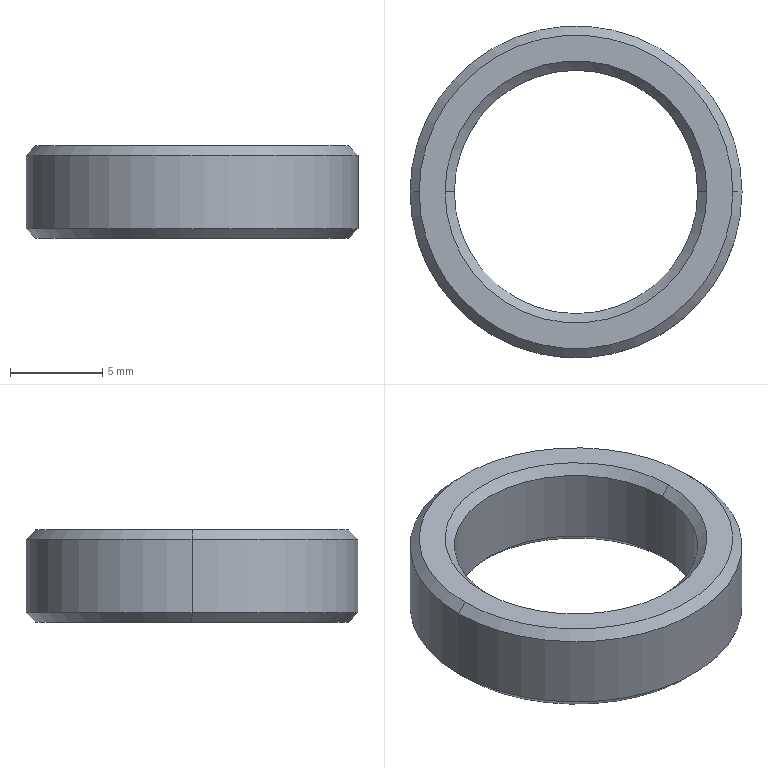Part | STEP file | 229H151427 Default | 1 solid | 14 faces | box 18 x 18 x 5 mm | volume 563.602 mm3 | cone 8 | cylinder 4 | plane 2 | commonest cylinder face diameters 13.2 x2 18 x2
STEP:
#1=CARTESIAN_POINT('',(-6.6,0.,4.5));
#2=VERTEX_POINT('',#1);
#3=CARTESIAN_POINT('',(6.6,0.,4.5));
#4=VERTEX_POINT('',#3);
#5=CARTESIAN_POINT('',(0.,0.,4.5));
#6=DIRECTION('',(0.,0.,1.));
#7=DIRECTION('',(1.,0.,0.));
#8=AXIS2_PLACEMENT_3D('',#5,#6,#7);
#9=CIRCLE('',#8,6.6);
#10=EDGE_CURVE('',#2,#4,#9,.T.);
#11=ORIENTED_EDGE('',*,*,#10,.F.);
#12=CARTESIAN_POINT('',(-7.1,0.,5.));
#13=VERTEX_POINT('',#12);
#14=CARTESIAN_POINT('',(-6.6,0.,4.5));
#15=DIRECTION('',(-0.7071,0.,0.7071));
#16=VECTOR('',#15,1000.);
#17=LINE('',#14,#16);
#18=EDGE_CURVE('',#2,#13,#17,.T.);
#19=ORIENTED_EDGE('',*,*,#18,.T.);
#20=CARTESIAN_POINT('',(7.1,0.,5.));
#21=VERTEX_POINT('',#20);
#22=CARTESIAN_POINT('',(0.,0.,5.));
#23=DIRECTION('',(0.,0.,-1.));
#24=DIRECTION('',(1.,0.,0.));
#25=AXIS2_PLACEMENT_3D('',#22,#23,#24);
#26=CIRCLE('',#25,7.1);
#27=EDGE_CURVE('',#21,#13,#26,.T.);
#28=ORIENTED_EDGE('',*,*,#27,.F.);
#29=CARTESIAN_POINT('',(6.6,0.,4.5));
#30=DIRECTION('',(0.7071,0.,0.7071));
#31=VECTOR('',#30,1000.);
#32=LINE('',#29,#31);
#33=EDGE_CURVE('',#4,#21,#32,.T.);
#34=ORIENTED_EDGE('',*,*,#33,.F.);
#35=EDGE_LOOP('',(#11,#19,#28,#34));
#36=FACE_OUTER_BOUND('',#35,.T.);
#37=CARTESIAN_POINT('',(0.,0.,4.5));
#38=DIRECTION('',(0.,0.,1.));
#39=DIRECTION('',(1.,0.,0.));
#40=AXIS2_PLACEMENT_3D('',#37,#38,#39);
#41=CONICAL_SURFACE('',#40,6.6,0.7854);
#42=ADVANCED_FACE('',(#36),#41,.F.);
#43=CARTESIAN_POINT('',(6.6,0.,0.5));
#44=VERTEX_POINT('',#43);
#45=CARTESIAN_POINT('',(-6.6,0.,0.5));
#46=VERTEX_POINT('',#45);
#47=CARTESIAN_POINT('',(0.,0.,0.5));
#48=DIRECTION('',(0.,0.,-1.));
#49=DIRECTION('',(1.,0.,0.));
#50=AXIS2_PLACEMENT_3D('',#47,#48,#49);
#51=CIRCLE('',#50,6.6);
#52=EDGE_CURVE('',#44,#46,#51,.T.);
#53=ORIENTED_EDGE('',*,*,#52,.F.);
#54=CARTESIAN_POINT('',(7.1,0.,0.));
#55=VERTEX_POINT('',#54);
#56=CARTESIAN_POINT('',(7.1,0.,0.));
#57=DIRECTION('',(0.7071,0.,-0.7071));
#58=VECTOR('',#57,1000.);
#59=LINE('',#56,#58);
#60=EDGE_CURVE('',#44,#55,#59,.T.);
#61=ORIENTED_EDGE('',*,*,#60,.T.);
#62=CARTESIAN_POINT('',(-7.1,0.,0.));
#63=VERTEX_POINT('',#62);
#64=CARTESIAN_POINT('',(0.,0.,0.));
#65=DIRECTION('',(0.,0.,1.));
#66=DIRECTION('',(1.,0.,0.));
#67=AXIS2_PLACEMENT_3D('',#64,#65,#66);
#68=CIRCLE('',#67,7.1);
#69=EDGE_CURVE('',#63,#55,#68,.T.);
#70=ORIENTED_EDGE('',*,*,#69,.F.);
#71=CARTESIAN_POINT('',(-7.1,0.,0.));
#72=DIRECTION('',(-0.7071,0.,-0.7071));
#73=VECTOR('',#72,1000.);
#74=LINE('',#71,#73);
#75=EDGE_CURVE('',#46,#63,#74,.T.);
#76=ORIENTED_EDGE('',*,*,#75,.F.);
#77=EDGE_LOOP('',(#53,#61,#70,#76));
#78=FACE_OUTER_BOUND('',#77,.T.);
#79=CARTESIAN_POINT('',(0.,0.,0.));
#80=DIRECTION('',(0.,0.,-1.));
#81=DIRECTION('',(-1.,0.,0.));
#82=AXIS2_PLACEMENT_3D('',#79,#80,#81);
#83=CONICAL_SURFACE('',#82,7.1,0.7854);
#84=ADVANCED_FACE('',(#78),#83,.F.);
#85=CARTESIAN_POINT('',(8.5,0.,5.));
#86=VERTEX_POINT('',#85);
#87=CARTESIAN_POINT('',(-8.5,0.,5.));
#88=VERTEX_POINT('',#87);
#89=CARTESIAN_POINT('',(0.,0.,5.));
#90=DIRECTION('',(0.,0.,1.));
#91=DIRECTION('',(1.,0.,0.));
#92=AXIS2_PLACEMENT_3D('',#89,#90,#91);
#93=CIRCLE('',#92,8.5);
#94=EDGE_CURVE('',#86,#88,#93,.T.);
#95=ORIENTED_EDGE('',*,*,#94,.F.);
#96=CARTESIAN_POINT('',(9.,0.,4.5));
#97=VERTEX_POINT('',#96);
#98=CARTESIAN_POINT('',(8.5,0.,5.));
#99=DIRECTION('',(0.7071,0.,-0.7071));
#100=VECTOR('',#99,1000.);
#101=LINE('',#98,#100);
#102=EDGE_CURVE('',#86,#97,#101,.T.);
#103=ORIENTED_EDGE('',*,*,#102,.T.);
#104=CARTESIAN_POINT('',(-9.,0.,4.5));
#105=VERTEX_POINT('',#104);
#106=CARTESIAN_POINT('',(0.,0.,4.5));
#107=DIRECTION('',(0.,0.,-1.));
#108=DIRECTION('',(1.,0.,0.));
#109=AXIS2_PLACEMENT_3D('',#106,#107,#108);
#110=CIRCLE('',#109,9.);
#111=EDGE_CURVE('',#105,#97,#110,.T.);
#112=ORIENTED_EDGE('',*,*,#111,.F.);
#113=CARTESIAN_POINT('',(-8.5,0.,5.));
#114=DIRECTION('',(-0.7071,0.,-0.7071));
#115=VECTOR('',#114,1000.);
#116=LINE('',#113,#115);
#117=EDGE_CURVE('',#88,#105,#116,.T.);
#118=ORIENTED_EDGE('',*,*,#117,.F.);
#119=EDGE_LOOP('',(#95,#103,#112,#118));
#120=FACE_OUTER_BOUND('',#119,.T.);
#121=CARTESIAN_POINT('',(0.,0.,5.));
#122=DIRECTION('',(0.,0.,-1.));
#123=DIRECTION('',(-1.,0.,0.));
#124=AXIS2_PLACEMENT_3D('',#121,#122,#123);
#125=CONICAL_SURFACE('',#124,8.5,0.7854);
#126=ADVANCED_FACE('',(#120),#125,.T.);
#127=CARTESIAN_POINT('',(-8.5,0.,0.));
#128=VERTEX_POINT('',#127);
#129=CARTESIAN_POINT('',(8.5,0.,0.));
#130=VERTEX_POINT('',#129);
#131=CARTESIAN_POINT('',(0.,0.,0.));
#132=DIRECTION('',(0.,0.,-1.));
#133=DIRECTION('',(1.,0.,0.));
#134=AXIS2_PLACEMENT_3D('',#131,#132,#133);
#135=CIRCLE('',#134,8.5);
#136=EDGE_CURVE('',#128,#130,#135,.T.);
#137=ORIENTED_EDGE('',*,*,#136,.F.);
#138=CARTESIAN_POINT('',(-9.,0.,0.5));
#139=VERTEX_POINT('',#138);
#140=CARTESIAN_POINT('',(-9.,0.,0.5));
#141=DIRECTION('',(-0.7071,0.,0.7071));
#142=VECTOR('',#141,1000.);
#143=LINE('',#140,#142);
#144=EDGE_CURVE('',#128,#139,#143,.T.);
#145=ORIENTED_EDGE('',*,*,#144,.T.);
#146=CARTESIAN_POINT('',(9.,0.,0.5));
#147=VERTEX_POINT('',#146);
#148=CARTESIAN_POINT('',(0.,0.,0.5));
#149=DIRECTION('',(0.,0.,1.));
#150=DIRECTION('',(1.,0.,0.));
#151=AXIS2_PLACEMENT_3D('',#148,#149,#150);
#152=CIRCLE('',#151,9.);
#153=EDGE_CURVE('',#147,#139,#152,.T.);
#154=ORIENTED_EDGE('',*,*,#153,.F.);
#155=CARTESIAN_POINT('',(9.,0.,0.5));
#156=DIRECTION('',(0.7071,0.,0.7071));
#157=VECTOR('',#156,1000.);
#158=LINE('',#155,#157);
#159=EDGE_CURVE('',#130,#147,#158,.T.);
#160=ORIENTED_EDGE('',*,*,#159,.F.);
#161=EDGE_LOOP('',(#137,#145,#154,#160));
#162=FACE_OUTER_BOUND('',#161,.T.);
#163=CARTESIAN_POINT('',(0.,0.,0.5));
#164=DIRECTION('',(0.,0.,1.));
#165=DIRECTION('',(1.,0.,0.));
#166=AXIS2_PLACEMENT_3D('',#163,#164,#165);
#167=CONICAL_SURFACE('',#166,9.,0.7854);
#168=ADVANCED_FACE('',(#162),#167,.T.);
#169=ORIENTED_EDGE('',*,*,#10,.T.);
#170=CARTESIAN_POINT('',(6.6,0.,5.));
#171=DIRECTION('',(0.,0.,-1.));
#172=VECTOR('',#171,1000.);
#173=LINE('',#170,#172);
#174=EDGE_CURVE('',#4,#44,#173,.T.);
#175=ORIENTED_EDGE('',*,*,#174,.T.);
#176=ORIENTED_EDGE('',*,*,#52,.T.);
#177=CARTESIAN_POINT('',(-6.6,0.,5.));
#178=DIRECTION('',(0.,0.,-1.));
#179=VECTOR('',#178,1000.);
#180=LINE('',#177,#179);
#181=EDGE_CURVE('',#2,#46,#180,.T.);
#182=ORIENTED_EDGE('',*,*,#181,.F.);
#183=EDGE_LOOP('',(#169,#175,#176,#182));
#184=FACE_OUTER_BOUND('',#183,.T.);
#185=CARTESIAN_POINT('',(0.,0.,5.));
#186=DIRECTION('',(0.,0.,-1.));
#187=DIRECTION('',(-1.,0.,0.));
#188=AXIS2_PLACEMENT_3D('',#185,#186,#187);
#189=CYLINDRICAL_SURFACE('',#188,6.6);
#190=ADVANCED_FACE('',(#184),#189,.F.);
#191=ORIENTED_EDGE('',*,*,#111,.T.);
#192=CARTESIAN_POINT('',(9.,0.,5.));
#193=DIRECTION('',(0.,0.,-1.));
#194=VECTOR('',#193,1000.);
#195=LINE('',#192,#194);
#196=EDGE_CURVE('',#97,#147,#195,.T.);
#197=ORIENTED_EDGE('',*,*,#196,.T.);
#198=ORIENTED_EDGE('',*,*,#153,.T.);
#199=CARTESIAN_POINT('',(-9.,0.,5.));
#200=DIRECTION('',(0.,0.,-1.));
#201=VECTOR('',#200,1000.);
#202=LINE('',#199,#201);
#203=EDGE_CURVE('',#105,#139,#202,.T.);
#204=ORIENTED_EDGE('',*,*,#203,.F.);
#205=EDGE_LOOP('',(#191,#197,#198,#204));
#206=FACE_OUTER_BOUND('',#205,.T.);
#207=CARTESIAN_POINT('',(0.,0.,5.));
#208=DIRECTION('',(0.,0.,-1.));
#209=DIRECTION('',(-1.,0.,0.));
#210=AXIS2_PLACEMENT_3D('',#207,#208,#209);
#211=CYLINDRICAL_SURFACE('',#210,9.);
#212=ADVANCED_FACE('',(#206),#211,.T.);
#213=ORIENTED_EDGE('',*,*,#27,.T.);
#214=CARTESIAN_POINT('',(0.,0.,5.));
#215=DIRECTION('',(0.,0.,-1.));
#216=DIRECTION('',(1.,0.,0.));
#217=AXIS2_PLACEMENT_3D('',#214,#215,#216);
#218=CIRCLE('',#217,7.1);
#219=EDGE_CURVE('',#13,#21,#218,.T.);
#220=ORIENTED_EDGE('',*,*,#219,.T.);
#221=EDGE_LOOP('',(#213,#220));
#222=FACE_BOUND('',#221,.T.);
#223=CARTESIAN_POINT('',(0.,0.,5.));
#224=DIRECTION('',(0.,0.,1.));
#225=DIRECTION('',(1.,0.,0.));
#226=AXIS2_PLACEMENT_3D('',#223,#224,#225);
#227=CIRCLE('',#226,8.5);
#228=EDGE_CURVE('',#88,#86,#227,.T.);
#229=ORIENTED_EDGE('',*,*,#228,.T.);
#230=ORIENTED_EDGE('',*,*,#94,.T.);
#231=EDGE_LOOP('',(#229,#230));
#232=FACE_OUTER_BOUND('',#231,.T.);
#233=CARTESIAN_POINT('',(0.,0.,5.));
#234=DIRECTION('',(0.,0.,1.));
#235=DIRECTION('',(1.,0.,0.));
#236=AXIS2_PLACEMENT_3D('',#233,#234,#235);
#237=PLANE('',#236);
#238=ADVANCED_FACE('',(#222,#232),#237,.T.);
#239=ORIENTED_EDGE('',*,*,#69,.T.);
#240=CARTESIAN_POINT('',(0.,0.,0.));
#241=DIRECTION('',(0.,0.,1.));
#242=DIRECTION('',(1.,0.,0.));
#243=AXIS2_PLACEMENT_3D('',#240,#241,#242);
#244=CIRCLE('',#243,7.1);
#245=EDGE_CURVE('',#55,#63,#244,.T.);
#246=ORIENTED_EDGE('',*,*,#245,.T.);
#247=EDGE_LOOP('',(#239,#246));
#248=FACE_BOUND('',#247,.T.);
#249=CARTESIAN_POINT('',(0.,0.,0.));
#250=DIRECTION('',(0.,0.,-1.));
#251=DIRECTION('',(1.,0.,0.));
#252=AXIS2_PLACEMENT_3D('',#249,#250,#251);
#253=CIRCLE('',#252,8.5);
#254=EDGE_CURVE('',#130,#128,#253,.T.);
#255=ORIENTED_EDGE('',*,*,#254,.T.);
#256=ORIENTED_EDGE('',*,*,#136,.T.);
#257=EDGE_LOOP('',(#255,#256));
#258=FACE_OUTER_BOUND('',#257,.T.);
#259=CARTESIAN_POINT('',(0.,0.,0.));
#260=DIRECTION('',(0.,0.,1.));
#261=DIRECTION('',(1.,0.,0.));
#262=AXIS2_PLACEMENT_3D('',#259,#260,#261);
#263=PLANE('',#262);
#264=ADVANCED_FACE('',(#248,#258),#263,.F.);
#265=ORIENTED_EDGE('',*,*,#196,.F.);
#266=CARTESIAN_POINT('',(0.,0.,4.5));
#267=DIRECTION('',(0.,0.,-1.));
#268=DIRECTION('',(1.,0.,0.));
#269=AXIS2_PLACEMENT_3D('',#266,#267,#268);
#270=CIRCLE('',#269,9.);
#271=EDGE_CURVE('',#97,#105,#270,.T.);
#272=ORIENTED_EDGE('',*,*,#271,.T.);
#273=ORIENTED_EDGE('',*,*,#203,.T.);
#274=CARTESIAN_POINT('',(0.,0.,0.5));
#275=DIRECTION('',(0.,0.,1.));
#276=DIRECTION('',(1.,0.,0.));
#277=AXIS2_PLACEMENT_3D('',#274,#275,#276);
#278=CIRCLE('',#277,9.);
#279=EDGE_CURVE('',#139,#147,#278,.T.);
#280=ORIENTED_EDGE('',*,*,#279,.T.);
#281=EDGE_LOOP('',(#265,#272,#273,#280));
#282=FACE_OUTER_BOUND('',#281,.T.);
#283=CARTESIAN_POINT('',(0.,0.,5.));
#284=DIRECTION('',(0.,0.,-1.));
#285=DIRECTION('',(-1.,0.,0.));
#286=AXIS2_PLACEMENT_3D('',#283,#284,#285);
#287=CYLINDRICAL_SURFACE('',#286,9.);
#288=ADVANCED_FACE('',(#282),#287,.T.);
#289=ORIENTED_EDGE('',*,*,#174,.F.);
#290=CARTESIAN_POINT('',(0.,0.,4.5));
#291=DIRECTION('',(0.,0.,1.));
#292=DIRECTION('',(1.,0.,0.));
#293=AXIS2_PLACEMENT_3D('',#290,#291,#292);
#294=CIRCLE('',#293,6.6);
#295=EDGE_CURVE('',#4,#2,#294,.T.);
#296=ORIENTED_EDGE('',*,*,#295,.T.);
#297=ORIENTED_EDGE('',*,*,#181,.T.);
#298=CARTESIAN_POINT('',(0.,0.,0.5));
#299=DIRECTION('',(0.,0.,-1.));
#300=DIRECTION('',(1.,0.,0.));
#301=AXIS2_PLACEMENT_3D('',#298,#299,#300);
#302=CIRCLE('',#301,6.6);
#303=EDGE_CURVE('',#46,#44,#302,.T.);
#304=ORIENTED_EDGE('',*,*,#303,.T.);
#305=EDGE_LOOP('',(#289,#296,#297,#304));
#306=FACE_OUTER_BOUND('',#305,.T.);
#307=CARTESIAN_POINT('',(0.,0.,5.));
#308=DIRECTION('',(0.,0.,-1.));
#309=DIRECTION('',(-1.,0.,0.));
#310=AXIS2_PLACEMENT_3D('',#307,#308,#309);
#311=CYLINDRICAL_SURFACE('',#310,6.6);
#312=ADVANCED_FACE('',(#306),#311,.F.);
#313=ORIENTED_EDGE('',*,*,#144,.F.);
#314=ORIENTED_EDGE('',*,*,#254,.F.);
#315=ORIENTED_EDGE('',*,*,#159,.T.);
#316=ORIENTED_EDGE('',*,*,#279,.F.);
#317=EDGE_LOOP('',(#313,#314,#315,#316));
#318=FACE_OUTER_BOUND('',#317,.T.);
#319=CARTESIAN_POINT('',(0.,0.,0.5));
#320=DIRECTION('',(0.,0.,1.));
#321=DIRECTION('',(1.,0.,0.));
#322=AXIS2_PLACEMENT_3D('',#319,#320,#321);
#323=CONICAL_SURFACE('',#322,9.,0.7854);
#324=ADVANCED_FACE('',(#318),#323,.T.);
#325=ORIENTED_EDGE('',*,*,#102,.F.);
#326=ORIENTED_EDGE('',*,*,#228,.F.);
#327=ORIENTED_EDGE('',*,*,#117,.T.);
#328=ORIENTED_EDGE('',*,*,#271,.F.);
#329=EDGE_LOOP('',(#325,#326,#327,#328));
#330=FACE_OUTER_BOUND('',#329,.T.);
#331=CARTESIAN_POINT('',(0.,0.,5.));
#332=DIRECTION('',(0.,0.,-1.));
#333=DIRECTION('',(-1.,0.,0.));
#334=AXIS2_PLACEMENT_3D('',#331,#332,#333);
#335=CONICAL_SURFACE('',#334,8.5,0.7854);
#336=ADVANCED_FACE('',(#330),#335,.T.);
#337=ORIENTED_EDGE('',*,*,#60,.F.);
#338=ORIENTED_EDGE('',*,*,#303,.F.);
#339=ORIENTED_EDGE('',*,*,#75,.T.);
#340=ORIENTED_EDGE('',*,*,#245,.F.);
#341=EDGE_LOOP('',(#337,#338,#339,#340));
#342=FACE_OUTER_BOUND('',#341,.T.);
#343=CARTESIAN_POINT('',(0.,0.,0.));
#344=DIRECTION('',(0.,0.,-1.));
#345=DIRECTION('',(-1.,0.,0.));
#346=AXIS2_PLACEMENT_3D('',#343,#344,#345);
#347=CONICAL_SURFACE('',#346,7.1,0.7854);
#348=ADVANCED_FACE('',(#342),#347,.F.);
#349=ORIENTED_EDGE('',*,*,#18,.F.);
#350=ORIENTED_EDGE('',*,*,#295,.F.);
#351=ORIENTED_EDGE('',*,*,#33,.T.);
#352=ORIENTED_EDGE('',*,*,#219,.F.);
#353=EDGE_LOOP('',(#349,#350,#351,#352));
#354=FACE_OUTER_BOUND('',#353,.T.);
#355=CARTESIAN_POINT('',(0.,0.,4.5));
#356=DIRECTION('',(0.,0.,1.));
#357=DIRECTION('',(1.,0.,0.));
#358=AXIS2_PLACEMENT_3D('',#355,#356,#357);
#359=CONICAL_SURFACE('',#358,6.6,0.7854);
#360=ADVANCED_FACE('',(#354),#359,.F.);
#361=CLOSED_SHELL('',(#42,#84,#126,#168,#190,#212,#238,#264,#288,#312,#324,#336,#348,#360));
#362=MANIFOLD_SOLID_BREP('',#361);
#363=CARTESIAN_POINT('',(0.,0.,0.));
#364=DIRECTION('',(0.,0.,1.));
#365=DIRECTION('',(1.,0.,0.));
#366=AXIS2_PLACEMENT_3D('',#363,#364,#365);
#367=(LENGTH_UNIT()NAMED_UNIT(*)SI_UNIT(.MILLI.,.METRE.));
#368=UNCERTAINTY_MEASURE_WITH_UNIT(LENGTH_MEASURE(0.00001),#367,'','');
#369=(NAMED_UNIT(*)PLANE_ANGLE_UNIT()SI_UNIT($,.RADIAN.));
#370=(NAMED_UNIT(*)SI_UNIT($,.STERADIAN.)SOLID_ANGLE_UNIT());
#371=(GEOMETRIC_REPRESENTATION_CONTEXT(3)GLOBAL_UNCERTAINTY_ASSIGNED_CONTEXT((#368))GLOBAL_UNIT_ASSIGNED_CONTEXT((#367,#369,#370))REPRESENTATION_CONTEXT('',''));
#372=ADVANCED_BREP_SHAPE_REPRESENTATION('',(#362,#366),#371);